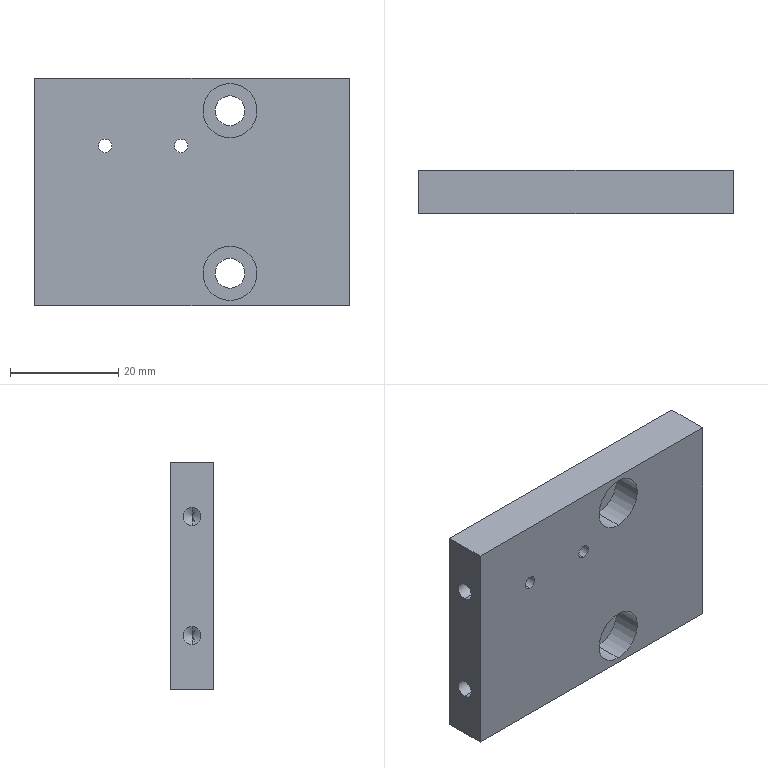Part | SolidWorks | features HoleWzd 3, Extrusion 1 | 1 solid | 28 faces | box 58 x 8 x 42 mm | volume 18259 mm3 | cylinder 16 | plane 8 | cone 4 | commonest cylinder face diameters 2.5 x4 3.3 x4 5.5 x4 10 x4
STEP:
#1=CARTESIAN_POINT('',(-16.,4.,9.75));
#2=VERTEX_POINT('',#1);
#3=CARTESIAN_POINT('',(-16.,4.,7.25));
#4=VERTEX_POINT('',#3);
#5=CARTESIAN_POINT('',(-16.,4.,8.5));
#6=DIRECTION('',(0.,-1.,0.));
#7=DIRECTION('',(0.,0.,-1.));
#8=AXIS2_PLACEMENT_3D('',#5,#6,#7);
#9=CIRCLE('',#8,1.25);
#10=EDGE_CURVE('',#2,#4,#9,.T.);
#11=ORIENTED_EDGE('',*,*,#10,.F.);
#12=CARTESIAN_POINT('',(-16.,-4.,9.75));
#13=VERTEX_POINT('',#12);
#14=CARTESIAN_POINT('',(-16.,-4.,9.75));
#15=DIRECTION('',(0.,-1.,0.));
#16=VECTOR('',#15,1000.);
#17=LINE('',#14,#16);
#18=EDGE_CURVE('',#2,#13,#17,.T.);
#19=ORIENTED_EDGE('',*,*,#18,.T.);
#20=CARTESIAN_POINT('',(-16.,-4.,7.25));
#21=VERTEX_POINT('',#20);
#22=CARTESIAN_POINT('',(-16.,-4.,8.5));
#23=DIRECTION('',(0.,-1.,0.));
#24=DIRECTION('',(0.,0.,-1.));
#25=AXIS2_PLACEMENT_3D('',#22,#23,#24);
#26=CIRCLE('',#25,1.25);
#27=EDGE_CURVE('',#13,#21,#26,.T.);
#28=ORIENTED_EDGE('',*,*,#27,.T.);
#29=CARTESIAN_POINT('',(-16.,-4.,7.25));
#30=DIRECTION('',(0.,-1.,0.));
#31=VECTOR('',#30,1000.);
#32=LINE('',#29,#31);
#33=EDGE_CURVE('',#4,#21,#32,.T.);
#34=ORIENTED_EDGE('',*,*,#33,.F.);
#35=EDGE_LOOP('',(#11,#19,#28,#34));
#36=FACE_OUTER_BOUND('',#35,.T.);
#37=CARTESIAN_POINT('',(-16.,-4.,8.5));
#38=DIRECTION('',(0.,-1.,0.));
#39=DIRECTION('',(0.,0.,-1.));
#40=AXIS2_PLACEMENT_3D('',#37,#38,#39);
#41=CYLINDRICAL_SURFACE('',#40,1.25);
#42=ADVANCED_FACE('',(#36),#41,.F.);
#43=CARTESIAN_POINT('',(-2.,4.,9.75));
#44=VERTEX_POINT('',#43);
#45=CARTESIAN_POINT('',(-2.,4.,7.25));
#46=VERTEX_POINT('',#45);
#47=CARTESIAN_POINT('',(-2.,4.,8.5));
#48=DIRECTION('',(0.,-1.,0.));
#49=DIRECTION('',(0.,0.,-1.));
#50=AXIS2_PLACEMENT_3D('',#47,#48,#49);
#51=CIRCLE('',#50,1.25);
#52=EDGE_CURVE('',#44,#46,#51,.T.);
#53=ORIENTED_EDGE('',*,*,#52,.F.);
#54=CARTESIAN_POINT('',(-2.,-4.,9.75));
#55=VERTEX_POINT('',#54);
#56=CARTESIAN_POINT('',(-2.,-4.,9.75));
#57=DIRECTION('',(0.,-1.,0.));
#58=VECTOR('',#57,1000.);
#59=LINE('',#56,#58);
#60=EDGE_CURVE('',#44,#55,#59,.T.);
#61=ORIENTED_EDGE('',*,*,#60,.T.);
#62=CARTESIAN_POINT('',(-2.,-4.,7.25));
#63=VERTEX_POINT('',#62);
#64=CARTESIAN_POINT('',(-2.,-4.,8.5));
#65=DIRECTION('',(0.,-1.,0.));
#66=DIRECTION('',(0.,0.,-1.));
#67=AXIS2_PLACEMENT_3D('',#64,#65,#66);
#68=CIRCLE('',#67,1.25);
#69=EDGE_CURVE('',#55,#63,#68,.T.);
#70=ORIENTED_EDGE('',*,*,#69,.T.);
#71=CARTESIAN_POINT('',(-2.,-4.,7.25));
#72=DIRECTION('',(0.,-1.,0.));
#73=VECTOR('',#72,1000.);
#74=LINE('',#71,#73);
#75=EDGE_CURVE('',#46,#63,#74,.T.);
#76=ORIENTED_EDGE('',*,*,#75,.F.);
#77=EDGE_LOOP('',(#53,#61,#70,#76));
#78=FACE_OUTER_BOUND('',#77,.T.);
#79=CARTESIAN_POINT('',(-2.,-4.,8.5));
#80=DIRECTION('',(0.,-1.,0.));
#81=DIRECTION('',(0.,0.,-1.));
#82=AXIS2_PLACEMENT_3D('',#79,#80,#81);
#83=CYLINDRICAL_SURFACE('',#82,1.25);
#84=ADVANCED_FACE('',(#78),#83,.F.);
#85=CARTESIAN_POINT('',(-18.9,0.,-12.65));
#86=VERTEX_POINT('',#85);
#87=CARTESIAN_POINT('',(-18.9,0.,-9.35));
#88=VERTEX_POINT('',#87);
#89=CARTESIAN_POINT('',(-18.9,0.,-11.));
#90=DIRECTION('',(-1.,0.,0.));
#91=DIRECTION('',(0.,0.,1.));
#92=AXIS2_PLACEMENT_3D('',#89,#90,#91);
#93=CIRCLE('',#92,1.65);
#94=EDGE_CURVE('',#86,#88,#93,.T.);
#95=ORIENTED_EDGE('',*,*,#94,.F.);
#96=CARTESIAN_POINT('',(-29.,0.,-12.65));
#97=VERTEX_POINT('',#96);
#98=CARTESIAN_POINT('',(-29.,0.,-12.65));
#99=DIRECTION('',(-1.,0.,0.));
#100=VECTOR('',#99,1000.);
#101=LINE('',#98,#100);
#102=EDGE_CURVE('',#86,#97,#101,.T.);
#103=ORIENTED_EDGE('',*,*,#102,.T.);
#104=CARTESIAN_POINT('',(-29.,0.,-9.35));
#105=VERTEX_POINT('',#104);
#106=CARTESIAN_POINT('',(-29.,0.,-11.));
#107=DIRECTION('',(-1.,0.,0.));
#108=DIRECTION('',(0.,0.,1.));
#109=AXIS2_PLACEMENT_3D('',#106,#107,#108);
#110=CIRCLE('',#109,1.65);
#111=EDGE_CURVE('',#97,#105,#110,.T.);
#112=ORIENTED_EDGE('',*,*,#111,.T.);
#113=CARTESIAN_POINT('',(-29.,0.,-9.35));
#114=DIRECTION('',(-1.,0.,0.));
#115=VECTOR('',#114,1000.);
#116=LINE('',#113,#115);
#117=EDGE_CURVE('',#88,#105,#116,.T.);
#118=ORIENTED_EDGE('',*,*,#117,.F.);
#119=EDGE_LOOP('',(#95,#103,#112,#118));
#120=FACE_OUTER_BOUND('',#119,.T.);
#121=CARTESIAN_POINT('',(-29.,0.,-11.));
#122=DIRECTION('',(-1.,0.,0.));
#123=DIRECTION('',(0.,0.,1.));
#124=AXIS2_PLACEMENT_3D('',#121,#122,#123);
#125=CYLINDRICAL_SURFACE('',#124,1.65);
#126=ADVANCED_FACE('',(#120),#125,.F.);
#127=CARTESIAN_POINT('',(-17.909,0.,-11.));
#128=VERTEX_POINT('',#127);
#129=CARTESIAN_POINT('',(-18.9,0.,-9.35));
#130=DIRECTION('',(-0.515,0.,0.8572));
#131=VECTOR('',#130,1000.);
#132=LINE('',#129,#131);
#133=EDGE_CURVE('',#128,#88,#132,.T.);
#134=ORIENTED_EDGE('',*,*,#133,.F.);
#135=CARTESIAN_POINT('',(-18.9,0.,-12.65));
#136=DIRECTION('',(-0.515,0.,-0.8572));
#137=VECTOR('',#136,1000.);
#138=LINE('',#135,#137);
#139=EDGE_CURVE('',#128,#86,#138,.T.);
#140=ORIENTED_EDGE('',*,*,#139,.T.);
#141=ORIENTED_EDGE('',*,*,#94,.T.);
#142=EDGE_LOOP('',(#134,#140,#141));
#143=FACE_OUTER_BOUND('',#142,.T.);
#144=CARTESIAN_POINT('',(-18.9,0.,-11.));
#145=DIRECTION('',(-1.,0.,0.));
#146=DIRECTION('',(0.,0.,1.));
#147=AXIS2_PLACEMENT_3D('',#144,#145,#146);
#148=CONICAL_SURFACE('',#147,1.65,1.03);
#149=ADVANCED_FACE('',(#143),#148,.F.);
#150=CARTESIAN_POINT('',(-18.9,0.,9.35));
#151=VERTEX_POINT('',#150);
#152=CARTESIAN_POINT('',(-18.9,0.,12.65));
#153=VERTEX_POINT('',#152);
#154=CARTESIAN_POINT('',(-18.9,0.,11.));
#155=DIRECTION('',(-1.,0.,0.));
#156=DIRECTION('',(0.,0.,1.));
#157=AXIS2_PLACEMENT_3D('',#154,#155,#156);
#158=CIRCLE('',#157,1.65);
#159=EDGE_CURVE('',#151,#153,#158,.T.);
#160=ORIENTED_EDGE('',*,*,#159,.F.);
#161=CARTESIAN_POINT('',(-29.,0.,9.35));
#162=VERTEX_POINT('',#161);
#163=CARTESIAN_POINT('',(-29.,0.,9.35));
#164=DIRECTION('',(-1.,0.,0.));
#165=VECTOR('',#164,1000.);
#166=LINE('',#163,#165);
#167=EDGE_CURVE('',#151,#162,#166,.T.);
#168=ORIENTED_EDGE('',*,*,#167,.T.);
#169=CARTESIAN_POINT('',(-29.,0.,12.65));
#170=VERTEX_POINT('',#169);
#171=CARTESIAN_POINT('',(-29.,0.,11.));
#172=DIRECTION('',(-1.,0.,0.));
#173=DIRECTION('',(0.,0.,1.));
#174=AXIS2_PLACEMENT_3D('',#171,#172,#173);
#175=CIRCLE('',#174,1.65);
#176=EDGE_CURVE('',#162,#170,#175,.T.);
#177=ORIENTED_EDGE('',*,*,#176,.T.);
#178=CARTESIAN_POINT('',(-29.,0.,12.65));
#179=DIRECTION('',(-1.,0.,0.));
#180=VECTOR('',#179,1000.);
#181=LINE('',#178,#180);
#182=EDGE_CURVE('',#153,#170,#181,.T.);
#183=ORIENTED_EDGE('',*,*,#182,.F.);
#184=EDGE_LOOP('',(#160,#168,#177,#183));
#185=FACE_OUTER_BOUND('',#184,.T.);
#186=CARTESIAN_POINT('',(-29.,0.,11.));
#187=DIRECTION('',(-1.,0.,0.));
#188=DIRECTION('',(0.,0.,1.));
#189=AXIS2_PLACEMENT_3D('',#186,#187,#188);
#190=CYLINDRICAL_SURFACE('',#189,1.65);
#191=ADVANCED_FACE('',(#185),#190,.F.);
#192=CARTESIAN_POINT('',(-17.909,0.,11.));
#193=VERTEX_POINT('',#192);
#194=CARTESIAN_POINT('',(-18.9,0.,12.65));
#195=DIRECTION('',(-0.515,0.,0.8572));
#196=VECTOR('',#195,1000.);
#197=LINE('',#194,#196);
#198=EDGE_CURVE('',#193,#153,#197,.T.);
#199=ORIENTED_EDGE('',*,*,#198,.F.);
#200=CARTESIAN_POINT('',(-18.9,0.,9.35));
#201=DIRECTION('',(-0.515,0.,-0.8572));
#202=VECTOR('',#201,1000.);
#203=LINE('',#200,#202);
#204=EDGE_CURVE('',#193,#151,#203,.T.);
#205=ORIENTED_EDGE('',*,*,#204,.T.);
#206=ORIENTED_EDGE('',*,*,#159,.T.);
#207=EDGE_LOOP('',(#199,#205,#206));
#208=FACE_OUTER_BOUND('',#207,.T.);
#209=CARTESIAN_POINT('',(-18.9,0.,11.));
#210=DIRECTION('',(-1.,0.,0.));
#211=DIRECTION('',(0.,0.,1.));
#212=AXIS2_PLACEMENT_3D('',#209,#210,#211);
#213=CONICAL_SURFACE('',#212,1.65,1.03);
#214=ADVANCED_FACE('',(#208),#213,.F.);
#215=CARTESIAN_POINT('',(7.,1.4,-10.));
#216=VERTEX_POINT('',#215);
#217=CARTESIAN_POINT('',(7.,1.4,-20.));
#218=VERTEX_POINT('',#217);
#219=CARTESIAN_POINT('',(7.,1.4,-15.));
#220=DIRECTION('',(0.,-1.,0.));
#221=DIRECTION('',(0.,0.,-1.));
#222=AXIS2_PLACEMENT_3D('',#219,#220,#221);
#223=CIRCLE('',#222,5.);
#224=EDGE_CURVE('',#216,#218,#223,.T.);
#225=ORIENTED_EDGE('',*,*,#224,.F.);
#226=CARTESIAN_POINT('',(7.,-4.,-10.));
#227=VERTEX_POINT('',#226);
#228=CARTESIAN_POINT('',(7.,-4.,-10.));
#229=DIRECTION('',(0.,-1.,0.));
#230=VECTOR('',#229,1000.);
#231=LINE('',#228,#230);
#232=EDGE_CURVE('',#216,#227,#231,.T.);
#233=ORIENTED_EDGE('',*,*,#232,.T.);
#234=CARTESIAN_POINT('',(7.,-4.,-20.));
#235=VERTEX_POINT('',#234);
#236=CARTESIAN_POINT('',(7.,-4.,-15.));
#237=DIRECTION('',(0.,-1.,0.));
#238=DIRECTION('',(0.,0.,-1.));
#239=AXIS2_PLACEMENT_3D('',#236,#237,#238);
#240=CIRCLE('',#239,5.);
#241=EDGE_CURVE('',#227,#235,#240,.T.);
#242=ORIENTED_EDGE('',*,*,#241,.T.);
#243=CARTESIAN_POINT('',(7.,-4.,-20.));
#244=DIRECTION('',(0.,-1.,0.));
#245=VECTOR('',#244,1000.);
#246=LINE('',#243,#245);
#247=EDGE_CURVE('',#218,#235,#246,.T.);
#248=ORIENTED_EDGE('',*,*,#247,.F.);
#249=EDGE_LOOP('',(#225,#233,#242,#248));
#250=FACE_OUTER_BOUND('',#249,.T.);
#251=CARTESIAN_POINT('',(7.,-4.,-15.));
#252=DIRECTION('',(0.,-1.,0.));
#253=DIRECTION('',(0.,0.,-1.));
#254=AXIS2_PLACEMENT_3D('',#251,#252,#253);
#255=CYLINDRICAL_SURFACE('',#254,5.);
#256=ADVANCED_FACE('',(#250),#255,.F.);
#257=CARTESIAN_POINT('',(7.,4.,-12.25));
#258=VERTEX_POINT('',#257);
#259=CARTESIAN_POINT('',(7.,4.,-17.75));
#260=VERTEX_POINT('',#259);
#261=CARTESIAN_POINT('',(7.,4.,-15.));
#262=DIRECTION('',(0.,-1.,0.));
#263=DIRECTION('',(0.,0.,-1.));
#264=AXIS2_PLACEMENT_3D('',#261,#262,#263);
#265=CIRCLE('',#264,2.75);
#266=EDGE_CURVE('',#258,#260,#265,.T.);
#267=ORIENTED_EDGE('',*,*,#266,.F.);
#268=CARTESIAN_POINT('',(7.,1.4,-12.25));
#269=VERTEX_POINT('',#268);
#270=CARTESIAN_POINT('',(7.,-4.,-12.25));
#271=DIRECTION('',(0.,-1.,0.));
#272=VECTOR('',#271,1000.);
#273=LINE('',#270,#272);
#274=EDGE_CURVE('',#258,#269,#273,.T.);
#275=ORIENTED_EDGE('',*,*,#274,.T.);
#276=CARTESIAN_POINT('',(7.,1.4,-17.75));
#277=VERTEX_POINT('',#276);
#278=CARTESIAN_POINT('',(7.,1.4,-15.));
#279=DIRECTION('',(0.,-1.,0.));
#280=DIRECTION('',(0.,0.,-1.));
#281=AXIS2_PLACEMENT_3D('',#278,#279,#280);
#282=CIRCLE('',#281,2.75);
#283=EDGE_CURVE('',#269,#277,#282,.T.);
#284=ORIENTED_EDGE('',*,*,#283,.T.);
#285=CARTESIAN_POINT('',(7.,-4.,-17.75));
#286=DIRECTION('',(0.,-1.,0.));
#287=VECTOR('',#286,1000.);
#288=LINE('',#285,#287);
#289=EDGE_CURVE('',#260,#277,#288,.T.);
#290=ORIENTED_EDGE('',*,*,#289,.F.);
#291=EDGE_LOOP('',(#267,#275,#284,#290));
#292=FACE_OUTER_BOUND('',#291,.T.);
#293=CARTESIAN_POINT('',(7.,-4.,-15.));
#294=DIRECTION('',(0.,-1.,0.));
#295=DIRECTION('',(0.,0.,-1.));
#296=AXIS2_PLACEMENT_3D('',#293,#294,#295);
#297=CYLINDRICAL_SURFACE('',#296,2.75);
#298=ADVANCED_FACE('',(#292),#297,.F.);
#299=CARTESIAN_POINT('',(7.,1.4,20.));
#300=VERTEX_POINT('',#299);
#301=CARTESIAN_POINT('',(7.,1.4,10.));
#302=VERTEX_POINT('',#301);
#303=CARTESIAN_POINT('',(7.,1.4,15.));
#304=DIRECTION('',(0.,-1.,0.));
#305=DIRECTION('',(0.,0.,-1.));
#306=AXIS2_PLACEMENT_3D('',#303,#304,#305);
#307=CIRCLE('',#306,5.);
#308=EDGE_CURVE('',#300,#302,#307,.T.);
#309=ORIENTED_EDGE('',*,*,#308,.F.);
#310=CARTESIAN_POINT('',(7.,-4.,20.));
#311=VERTEX_POINT('',#310);
#312=CARTESIAN_POINT('',(7.,-4.,20.));
#313=DIRECTION('',(0.,-1.,0.));
#314=VECTOR('',#313,1000.);
#315=LINE('',#312,#314);
#316=EDGE_CURVE('',#300,#311,#315,.T.);
#317=ORIENTED_EDGE('',*,*,#316,.T.);
#318=CARTESIAN_POINT('',(7.,-4.,10.));
#319=VERTEX_POINT('',#318);
#320=CARTESIAN_POINT('',(7.,-4.,15.));
#321=DIRECTION('',(0.,-1.,0.));
#322=DIRECTION('',(0.,0.,-1.));
#323=AXIS2_PLACEMENT_3D('',#320,#321,#322);
#324=CIRCLE('',#323,5.);
#325=EDGE_CURVE('',#311,#319,#324,.T.);
#326=ORIENTED_EDGE('',*,*,#325,.T.);
#327=CARTESIAN_POINT('',(7.,-4.,10.));
#328=DIRECTION('',(0.,-1.,0.));
#329=VECTOR('',#328,1000.);
#330=LINE('',#327,#329);
#331=EDGE_CURVE('',#302,#319,#330,.T.);
#332=ORIENTED_EDGE('',*,*,#331,.F.);
#333=EDGE_LOOP('',(#309,#317,#326,#332));
#334=FACE_OUTER_BOUND('',#333,.T.);
#335=CARTESIAN_POINT('',(7.,-4.,15.));
#336=DIRECTION('',(0.,-1.,0.));
#337=DIRECTION('',(0.,0.,-1.));
#338=AXIS2_PLACEMENT_3D('',#335,#336,#337);
#339=CYLINDRICAL_SURFACE('',#338,5.);
#340=ADVANCED_FACE('',(#334),#339,.F.);
#341=CARTESIAN_POINT('',(7.,4.,17.75));
#342=VERTEX_POINT('',#341);
#343=CARTESIAN_POINT('',(7.,4.,12.25));
#344=VERTEX_POINT('',#343);
#345=CARTESIAN_POINT('',(7.,4.,15.));
#346=DIRECTION('',(0.,-1.,0.));
#347=DIRECTION('',(0.,0.,-1.));
#348=AXIS2_PLACEMENT_3D('',#345,#346,#347);
#349=CIRCLE('',#348,2.75);
#350=EDGE_CURVE('',#342,#344,#349,.T.);
#351=ORIENTED_EDGE('',*,*,#350,.F.);
#352=CARTESIAN_POINT('',(7.,1.4,17.75));
#353=VERTEX_POINT('',#352);
#354=CARTESIAN_POINT('',(7.,-4.,17.75));
#355=DIRECTION('',(0.,-1.,0.));
#356=VECTOR('',#355,1000.);
#357=LINE('',#354,#356);
#358=EDGE_CURVE('',#342,#353,#357,.T.);
#359=ORIENTED_EDGE('',*,*,#358,.T.);
#360=CARTESIAN_POINT('',(7.,1.4,12.25));
#361=VERTEX_POINT('',#360);
#362=CARTESIAN_POINT('',(7.,1.4,15.));
#363=DIRECTION('',(0.,-1.,0.));
#364=DIRECTION('',(0.,0.,-1.));
#365=AXIS2_PLACEMENT_3D('',#362,#363,#364);
#366=CIRCLE('',#365,2.75);
#367=EDGE_CURVE('',#353,#361,#366,.T.);
#368=ORIENTED_EDGE('',*,*,#367,.T.);
#369=CARTESIAN_POINT('',(7.,-4.,12.25));
#370=DIRECTION('',(0.,-1.,0.));
#371=VECTOR('',#370,1000.);
#372=LINE('',#369,#371);
#373=EDGE_CURVE('',#344,#361,#372,.T.);
#374=ORIENTED_EDGE('',*,*,#373,.F.);
#375=EDGE_LOOP('',(#351,#359,#368,#374));
#376=FACE_OUTER_BOUND('',#375,.T.);
#377=CARTESIAN_POINT('',(7.,-4.,15.));
#378=DIRECTION('',(0.,-1.,0.));
#379=DIRECTION('',(0.,0.,-1.));
#380=AXIS2_PLACEMENT_3D('',#377,#378,#379);
#381=CYLINDRICAL_SURFACE('',#380,2.75);
#382=ADVANCED_FACE('',(#376),#381,.F.);
#383=CARTESIAN_POINT('',(29.,-4.,21.));
#384=VERTEX_POINT('',#383);
#385=CARTESIAN_POINT('',(29.,-4.,-21.));
#386=VERTEX_POINT('',#385);
#387=CARTESIAN_POINT('',(29.,-4.,-21.));
#388=DIRECTION('',(0.,0.,-1.));
#389=VECTOR('',#388,1000.);
#390=LINE('',#387,#389);
#391=EDGE_CURVE('',#384,#386,#390,.T.);
#392=ORIENTED_EDGE('',*,*,#391,.T.);
#393=CARTESIAN_POINT('',(29.,4.,-21.));
#394=VERTEX_POINT('',#393);
#395=CARTESIAN_POINT('',(29.,4.,-21.));
#396=DIRECTION('',(0.,-1.,0.));
#397=VECTOR('',#396,1000.);
#398=LINE('',#395,#397);
#399=EDGE_CURVE('',#394,#386,#398,.T.);
#400=ORIENTED_EDGE('',*,*,#399,.F.);
#401=CARTESIAN_POINT('',(29.,4.,21.));
#402=VERTEX_POINT('',#401);
#403=CARTESIAN_POINT('',(29.,4.,-21.));
#404=DIRECTION('',(0.,0.,-1.));
#405=VECTOR('',#404,1000.);
#406=LINE('',#403,#405);
#407=EDGE_CURVE('',#402,#394,#406,.T.);
#408=ORIENTED_EDGE('',*,*,#407,.F.);
#409=CARTESIAN_POINT('',(29.,4.,21.));
#410=DIRECTION('',(0.,-1.,0.));
#411=VECTOR('',#410,1000.);
#412=LINE('',#409,#411);
#413=EDGE_CURVE('',#402,#384,#412,.T.);
#414=ORIENTED_EDGE('',*,*,#413,.T.);
#415=EDGE_LOOP('',(#392,#400,#408,#414));
#416=FACE_OUTER_BOUND('',#415,.T.);
#417=CARTESIAN_POINT('',(29.,4.,-21.));
#418=DIRECTION('',(-1.,0.,0.));
#419=DIRECTION('',(0.,0.,1.));
#420=AXIS2_PLACEMENT_3D('',#417,#418,#419);
#421=PLANE('',#420);
#422=ADVANCED_FACE('',(#416),#421,.F.);
#423=CARTESIAN_POINT('',(-29.,-4.,-21.));
#424=VERTEX_POINT('',#423);
#425=CARTESIAN_POINT('',(-29.,-4.,-21.));
#426=DIRECTION('',(-1.,0.,0.));
#427=VECTOR('',#426,1000.);
#428=LINE('',#425,#427);
#429=EDGE_CURVE('',#386,#424,#428,.T.);
#430=ORIENTED_EDGE('',*,*,#429,.T.);
#431=CARTESIAN_POINT('',(-29.,4.,-21.));
#432=VERTEX_POINT('',#431);
#433=CARTESIAN_POINT('',(-29.,4.,-21.));
#434=DIRECTION('',(0.,-1.,0.));
#435=VECTOR('',#434,1000.);
#436=LINE('',#433,#435);
#437=EDGE_CURVE('',#432,#424,#436,.T.);
#438=ORIENTED_EDGE('',*,*,#437,.F.);
#439=CARTESIAN_POINT('',(-29.,4.,-21.));
#440=DIRECTION('',(-1.,0.,0.));
#441=VECTOR('',#440,1000.);
#442=LINE('',#439,#441);
#443=EDGE_CURVE('',#394,#432,#442,.T.);
#444=ORIENTED_EDGE('',*,*,#443,.F.);
#445=ORIENTED_EDGE('',*,*,#399,.T.);
#446=EDGE_LOOP('',(#430,#438,#444,#445));
#447=FACE_OUTER_BOUND('',#446,.T.);
#448=CARTESIAN_POINT('',(-29.,4.,-21.));
#449=DIRECTION('',(0.,0.,1.));
#450=DIRECTION('',(1.,0.,0.));
#451=AXIS2_PLACEMENT_3D('',#448,#449,#450);
#452=PLANE('',#451);
#453=ADVANCED_FACE('',(#447),#452,.F.);
#454=CARTESIAN_POINT('',(-29.,0.,-11.));
#455=DIRECTION('',(-1.,0.,0.));
#456=DIRECTION('',(0.,0.,1.));
#457=AXIS2_PLACEMENT_3D('',#454,#455,#456);
#458=CIRCLE('',#457,1.65);
#459=EDGE_CURVE('',#105,#97,#458,.T.);
#460=ORIENTED_EDGE('',*,*,#459,.F.);
#461=ORIENTED_EDGE('',*,*,#111,.F.);
#462=EDGE_LOOP('',(#460,#461));
#463=FACE_BOUND('',#462,.T.);
#464=CARTESIAN_POINT('',(-29.,0.,11.));
#465=DIRECTION('',(-1.,0.,0.));
#466=DIRECTION('',(0.,0.,1.));
#467=AXIS2_PLACEMENT_3D('',#464,#465,#466);
#468=CIRCLE('',#467,1.65);
#469=EDGE_CURVE('',#170,#162,#468,.T.);
#470=ORIENTED_EDGE('',*,*,#469,.F.);
#471=ORIENTED_EDGE('',*,*,#176,.F.);
#472=EDGE_LOOP('',(#470,#471));
#473=FACE_BOUND('',#472,.T.);
#474=CARTESIAN_POINT('',(-29.,-4.,21.));
#475=VERTEX_POINT('',#474);
#476=CARTESIAN_POINT('',(-29.,-4.,-21.));
#477=DIRECTION('',(0.,0.,1.));
#478=VECTOR('',#477,1000.);
#479=LINE('',#476,#478);
#480=EDGE_CURVE('',#424,#475,#479,.T.);
#481=ORIENTED_EDGE('',*,*,#480,.T.);
#482=CARTESIAN_POINT('',(-29.,4.,21.));
#483=VERTEX_POINT('',#482);
#484=CARTESIAN_POINT('',(-29.,4.,21.));
#485=DIRECTION('',(0.,-1.,0.));
#486=VECTOR('',#485,1000.);
#487=LINE('',#484,#486);
#488=EDGE_CURVE('',#483,#475,#487,.T.);
#489=ORIENTED_EDGE('',*,*,#488,.F.);
#490=CARTESIAN_POINT('',(-29.,4.,-21.));
#491=DIRECTION('',(0.,0.,1.));
#492=VECTOR('',#491,1000.);
#493=LINE('',#490,#492);
#494=EDGE_CURVE('',#432,#483,#493,.T.);
#495=ORIENTED_EDGE('',*,*,#494,.F.);
#496=ORIENTED_EDGE('',*,*,#437,.T.);
#497=EDGE_LOOP('',(#481,#489,#495,#496));
#498=FACE_OUTER_BOUND('',#497,.T.);
#499=CARTESIAN_POINT('',(-29.,4.,-21.));
#500=DIRECTION('',(1.,0.,0.));
#501=DIRECTION('',(0.,0.,-1.));
#502=AXIS2_PLACEMENT_3D('',#499,#500,#501);
#503=PLANE('',#502);
#504=ADVANCED_FACE('',(#463,#473,#498),#503,.F.);
#505=CARTESIAN_POINT('',(-29.,-4.,21.));
#506=DIRECTION('',(1.,0.,0.));
#507=VECTOR('',#506,1000.);
#508=LINE('',#505,#507);
#509=EDGE_CURVE('',#475,#384,#508,.T.);
#510=ORIENTED_EDGE('',*,*,#509,.T.);
#511=ORIENTED_EDGE('',*,*,#413,.F.);
#512=CARTESIAN_POINT('',(-29.,4.,21.));
#513=DIRECTION('',(1.,0.,0.));
#514=VECTOR('',#513,1000.);
#515=LINE('',#512,#514);
#516=EDGE_CURVE('',#483,#402,#515,.T.);
#517=ORIENTED_EDGE('',*,*,#516,.F.);
#518=ORIENTED_EDGE('',*,*,#488,.T.);
#519=EDGE_LOOP('',(#510,#511,#517,#518));
#520=FACE_OUTER_BOUND('',#519,.T.);
#521=CARTESIAN_POINT('',(-29.,4.,21.));
#522=DIRECTION('',(0.,0.,-1.));
#523=DIRECTION('',(-1.,0.,0.));
#524=AXIS2_PLACEMENT_3D('',#521,#522,#523);
#525=PLANE('',#524);
#526=ADVANCED_FACE('',(#520),#525,.F.);
#527=CARTESIAN_POINT('',(-16.,4.,8.5));
#528=DIRECTION('',(0.,-1.,0.));
#529=DIRECTION('',(0.,0.,-1.));
#530=AXIS2_PLACEMENT_3D('',#527,#528,#529);
#531=CIRCLE('',#530,1.25);
#532=EDGE_CURVE('',#4,#2,#531,.T.);
#533=ORIENTED_EDGE('',*,*,#532,.T.);
#534=ORIENTED_EDGE('',*,*,#10,.T.);
#535=EDGE_LOOP('',(#533,#534));
#536=FACE_BOUND('',#535,.T.);
#537=CARTESIAN_POINT('',(-2.,4.,8.5));
#538=DIRECTION('',(0.,-1.,0.));
#539=DIRECTION('',(0.,0.,-1.));
#540=AXIS2_PLACEMENT_3D('',#537,#538,#539);
#541=CIRCLE('',#540,1.25);
#542=EDGE_CURVE('',#46,#44,#541,.T.);
#543=ORIENTED_EDGE('',*,*,#542,.T.);
#544=ORIENTED_EDGE('',*,*,#52,.T.);
#545=EDGE_LOOP('',(#543,#544));
#546=FACE_BOUND('',#545,.T.);
#547=CARTESIAN_POINT('',(7.,4.,-15.));
#548=DIRECTION('',(0.,-1.,0.));
#549=DIRECTION('',(0.,0.,-1.));
#550=AXIS2_PLACEMENT_3D('',#547,#548,#549);
#551=CIRCLE('',#550,2.75);
#552=EDGE_CURVE('',#260,#258,#551,.T.);
#553=ORIENTED_EDGE('',*,*,#552,.T.);
#554=ORIENTED_EDGE('',*,*,#266,.T.);
#555=EDGE_LOOP('',(#553,#554));
#556=FACE_BOUND('',#555,.T.);
#557=CARTESIAN_POINT('',(7.,4.,15.));
#558=DIRECTION('',(0.,-1.,0.));
#559=DIRECTION('',(0.,0.,-1.));
#560=AXIS2_PLACEMENT_3D('',#557,#558,#559);
#561=CIRCLE('',#560,2.75);
#562=EDGE_CURVE('',#344,#342,#561,.T.);
#563=ORIENTED_EDGE('',*,*,#562,.T.);
#564=ORIENTED_EDGE('',*,*,#350,.T.);
#565=EDGE_LOOP('',(#563,#564));
#566=FACE_BOUND('',#565,.T.);
#567=ORIENTED_EDGE('',*,*,#407,.T.);
#568=ORIENTED_EDGE('',*,*,#443,.T.);
#569=ORIENTED_EDGE('',*,*,#494,.T.);
#570=ORIENTED_EDGE('',*,*,#516,.T.);
#571=EDGE_LOOP('',(#567,#568,#569,#570));
#572=FACE_OUTER_BOUND('',#571,.T.);
#573=CARTESIAN_POINT('',(0.,4.,0.));
#574=DIRECTION('',(0.,1.,0.));
#575=DIRECTION('',(0.,0.,1.));
#576=AXIS2_PLACEMENT_3D('',#573,#574,#575);
#577=PLANE('',#576);
#578=ADVANCED_FACE('',(#536,#546,#556,#566,#572),#577,.T.);
#579=CARTESIAN_POINT('',(-16.,-4.,8.5));
#580=DIRECTION('',(0.,-1.,0.));
#581=DIRECTION('',(0.,0.,-1.));
#582=AXIS2_PLACEMENT_3D('',#579,#580,#581);
#583=CIRCLE('',#582,1.25);
#584=EDGE_CURVE('',#21,#13,#583,.T.);
#585=ORIENTED_EDGE('',*,*,#584,.F.);
#586=ORIENTED_EDGE('',*,*,#27,.F.);
#587=EDGE_LOOP('',(#585,#586));
#588=FACE_BOUND('',#587,.T.);
#589=CARTESIAN_POINT('',(-2.,-4.,8.5));
#590=DIRECTION('',(0.,-1.,0.));
#591=DIRECTION('',(0.,0.,-1.));
#592=AXIS2_PLACEMENT_3D('',#589,#590,#591);
#593=CIRCLE('',#592,1.25);
#594=EDGE_CURVE('',#63,#55,#593,.T.);
#595=ORIENTED_EDGE('',*,*,#594,.F.);
#596=ORIENTED_EDGE('',*,*,#69,.F.);
#597=EDGE_LOOP('',(#595,#596));
#598=FACE_BOUND('',#597,.T.);
#599=CARTESIAN_POINT('',(7.,-4.,-15.));
#600=DIRECTION('',(0.,-1.,0.));
#601=DIRECTION('',(0.,0.,-1.));
#602=AXIS2_PLACEMENT_3D('',#599,#600,#601);
#603=CIRCLE('',#602,5.);
#604=EDGE_CURVE('',#235,#227,#603,.T.);
#605=ORIENTED_EDGE('',*,*,#604,.F.);
#606=ORIENTED_EDGE('',*,*,#241,.F.);
#607=EDGE_LOOP('',(#605,#606));
#608=FACE_BOUND('',#607,.T.);
#609=CARTESIAN_POINT('',(7.,-4.,15.));
#610=DIRECTION('',(0.,-1.,0.));
#611=DIRECTION('',(0.,0.,-1.));
#612=AXIS2_PLACEMENT_3D('',#609,#610,#611);
#613=CIRCLE('',#612,5.);
#614=EDGE_CURVE('',#319,#311,#613,.T.);
#615=ORIENTED_EDGE('',*,*,#614,.F.);
#616=ORIENTED_EDGE('',*,*,#325,.F.);
#617=EDGE_LOOP('',(#615,#616));
#618=FACE_BOUND('',#617,.T.);
#619=ORIENTED_EDGE('',*,*,#391,.F.);
#620=ORIENTED_EDGE('',*,*,#509,.F.);
#621=ORIENTED_EDGE('',*,*,#480,.F.);
#622=ORIENTED_EDGE('',*,*,#429,.F.);
#623=EDGE_LOOP('',(#619,#620,#621,#622));
#624=FACE_OUTER_BOUND('',#623,.T.);
#625=CARTESIAN_POINT('',(0.,-4.,0.));
#626=DIRECTION('',(0.,1.,0.));
#627=DIRECTION('',(0.,0.,1.));
#628=AXIS2_PLACEMENT_3D('',#625,#626,#627);
#629=PLANE('',#628);
#630=ADVANCED_FACE('',(#588,#598,#608,#618,#624),#629,.F.);
#631=ORIENTED_EDGE('',*,*,#358,.F.);
#632=ORIENTED_EDGE('',*,*,#562,.F.);
#633=ORIENTED_EDGE('',*,*,#373,.T.);
#634=CARTESIAN_POINT('',(7.,1.4,15.));
#635=DIRECTION('',(0.,-1.,0.));
#636=DIRECTION('',(0.,0.,-1.));
#637=AXIS2_PLACEMENT_3D('',#634,#635,#636);
#638=CIRCLE('',#637,2.75);
#639=EDGE_CURVE('',#361,#353,#638,.T.);
#640=ORIENTED_EDGE('',*,*,#639,.T.);
#641=EDGE_LOOP('',(#631,#632,#633,#640));
#642=FACE_OUTER_BOUND('',#641,.T.);
#643=CARTESIAN_POINT('',(7.,-4.,15.));
#644=DIRECTION('',(0.,-1.,0.));
#645=DIRECTION('',(0.,0.,-1.));
#646=AXIS2_PLACEMENT_3D('',#643,#644,#645);
#647=CYLINDRICAL_SURFACE('',#646,2.75);
#648=ADVANCED_FACE('',(#642),#647,.F.);
#649=ORIENTED_EDGE('',*,*,#639,.F.);
#650=ORIENTED_EDGE('',*,*,#367,.F.);
#651=EDGE_LOOP('',(#649,#650));
#652=FACE_BOUND('',#651,.T.);
#653=CARTESIAN_POINT('',(7.,1.4,15.));
#654=DIRECTION('',(0.,-1.,0.));
#655=DIRECTION('',(0.,0.,-1.));
#656=AXIS2_PLACEMENT_3D('',#653,#654,#655);
#657=CIRCLE('',#656,5.);
#658=EDGE_CURVE('',#302,#300,#657,.T.);
#659=ORIENTED_EDGE('',*,*,#658,.T.);
#660=ORIENTED_EDGE('',*,*,#308,.T.);
#661=EDGE_LOOP('',(#659,#660));
#662=FACE_OUTER_BOUND('',#661,.T.);
#663=CARTESIAN_POINT('',(9.75,1.4,15.));
#664=DIRECTION('',(0.,1.,0.));
#665=DIRECTION('',(0.,0.,1.));
#666=AXIS2_PLACEMENT_3D('',#663,#664,#665);
#667=PLANE('',#666);
#668=ADVANCED_FACE('',(#652,#662),#667,.F.);
#669=ORIENTED_EDGE('',*,*,#316,.F.);
#670=ORIENTED_EDGE('',*,*,#658,.F.);
#671=ORIENTED_EDGE('',*,*,#331,.T.);
#672=ORIENTED_EDGE('',*,*,#614,.T.);
#673=EDGE_LOOP('',(#669,#670,#671,#672));
#674=FACE_OUTER_BOUND('',#673,.T.);
#675=CARTESIAN_POINT('',(7.,-4.,15.));
#676=DIRECTION('',(0.,-1.,0.));
#677=DIRECTION('',(0.,0.,-1.));
#678=AXIS2_PLACEMENT_3D('',#675,#676,#677);
#679=CYLINDRICAL_SURFACE('',#678,5.);
#680=ADVANCED_FACE('',(#674),#679,.F.);
#681=ORIENTED_EDGE('',*,*,#274,.F.);
#682=ORIENTED_EDGE('',*,*,#552,.F.);
#683=ORIENTED_EDGE('',*,*,#289,.T.);
#684=CARTESIAN_POINT('',(7.,1.4,-15.));
#685=DIRECTION('',(0.,-1.,0.));
#686=DIRECTION('',(0.,0.,-1.));
#687=AXIS2_PLACEMENT_3D('',#684,#685,#686);
#688=CIRCLE('',#687,2.75);
#689=EDGE_CURVE('',#277,#269,#688,.T.);
#690=ORIENTED_EDGE('',*,*,#689,.T.);
#691=EDGE_LOOP('',(#681,#682,#683,#690));
#692=FACE_OUTER_BOUND('',#691,.T.);
#693=CARTESIAN_POINT('',(7.,-4.,-15.));
#694=DIRECTION('',(0.,-1.,0.));
#695=DIRECTION('',(0.,0.,-1.));
#696=AXIS2_PLACEMENT_3D('',#693,#694,#695);
#697=CYLINDRICAL_SURFACE('',#696,2.75);
#698=ADVANCED_FACE('',(#692),#697,.F.);
#699=ORIENTED_EDGE('',*,*,#689,.F.);
#700=ORIENTED_EDGE('',*,*,#283,.F.);
#701=EDGE_LOOP('',(#699,#700));
#702=FACE_BOUND('',#701,.T.);
#703=CARTESIAN_POINT('',(7.,1.4,-15.));
#704=DIRECTION('',(0.,-1.,0.));
#705=DIRECTION('',(0.,0.,-1.));
#706=AXIS2_PLACEMENT_3D('',#703,#704,#705);
#707=CIRCLE('',#706,5.);
#708=EDGE_CURVE('',#218,#216,#707,.T.);
#709=ORIENTED_EDGE('',*,*,#708,.T.);
#710=ORIENTED_EDGE('',*,*,#224,.T.);
#711=EDGE_LOOP('',(#709,#710));
#712=FACE_OUTER_BOUND('',#711,.T.);
#713=CARTESIAN_POINT('',(9.75,1.4,-15.));
#714=DIRECTION('',(0.,1.,0.));
#715=DIRECTION('',(0.,0.,1.));
#716=AXIS2_PLACEMENT_3D('',#713,#714,#715);
#717=PLANE('',#716);
#718=ADVANCED_FACE('',(#702,#712),#717,.F.);
#719=ORIENTED_EDGE('',*,*,#232,.F.);
#720=ORIENTED_EDGE('',*,*,#708,.F.);
#721=ORIENTED_EDGE('',*,*,#247,.T.);
#722=ORIENTED_EDGE('',*,*,#604,.T.);
#723=EDGE_LOOP('',(#719,#720,#721,#722));
#724=FACE_OUTER_BOUND('',#723,.T.);
#725=CARTESIAN_POINT('',(7.,-4.,-15.));
#726=DIRECTION('',(0.,-1.,0.));
#727=DIRECTION('',(0.,0.,-1.));
#728=AXIS2_PLACEMENT_3D('',#725,#726,#727);
#729=CYLINDRICAL_SURFACE('',#728,5.);
#730=ADVANCED_FACE('',(#724),#729,.F.);
#731=ORIENTED_EDGE('',*,*,#204,.F.);
#732=ORIENTED_EDGE('',*,*,#198,.T.);
#733=CARTESIAN_POINT('',(-18.9,0.,11.));
#734=DIRECTION('',(-1.,0.,0.));
#735=DIRECTION('',(0.,0.,1.));
#736=AXIS2_PLACEMENT_3D('',#733,#734,#735);
#737=CIRCLE('',#736,1.65);
#738=EDGE_CURVE('',#153,#151,#737,.T.);
#739=ORIENTED_EDGE('',*,*,#738,.T.);
#740=EDGE_LOOP('',(#731,#732,#739));
#741=FACE_OUTER_BOUND('',#740,.T.);
#742=CARTESIAN_POINT('',(-18.9,0.,11.));
#743=DIRECTION('',(-1.,0.,0.));
#744=DIRECTION('',(0.,0.,1.));
#745=AXIS2_PLACEMENT_3D('',#742,#743,#744);
#746=CONICAL_SURFACE('',#745,1.65,1.03);
#747=ADVANCED_FACE('',(#741),#746,.F.);
#748=ORIENTED_EDGE('',*,*,#167,.F.);
#749=ORIENTED_EDGE('',*,*,#738,.F.);
#750=ORIENTED_EDGE('',*,*,#182,.T.);
#751=ORIENTED_EDGE('',*,*,#469,.T.);
#752=EDGE_LOOP('',(#748,#749,#750,#751));
#753=FACE_OUTER_BOUND('',#752,.T.);
#754=CARTESIAN_POINT('',(-29.,0.,11.));
#755=DIRECTION('',(-1.,0.,0.));
#756=DIRECTION('',(0.,0.,1.));
#757=AXIS2_PLACEMENT_3D('',#754,#755,#756);
#758=CYLINDRICAL_SURFACE('',#757,1.65);
#759=ADVANCED_FACE('',(#753),#758,.F.);
#760=ORIENTED_EDGE('',*,*,#139,.F.);
#761=ORIENTED_EDGE('',*,*,#133,.T.);
#762=CARTESIAN_POINT('',(-18.9,0.,-11.));
#763=DIRECTION('',(-1.,0.,0.));
#764=DIRECTION('',(0.,0.,1.));
#765=AXIS2_PLACEMENT_3D('',#762,#763,#764);
#766=CIRCLE('',#765,1.65);
#767=EDGE_CURVE('',#88,#86,#766,.T.);
#768=ORIENTED_EDGE('',*,*,#767,.T.);
#769=EDGE_LOOP('',(#760,#761,#768));
#770=FACE_OUTER_BOUND('',#769,.T.);
#771=CARTESIAN_POINT('',(-18.9,0.,-11.));
#772=DIRECTION('',(-1.,0.,0.));
#773=DIRECTION('',(0.,0.,1.));
#774=AXIS2_PLACEMENT_3D('',#771,#772,#773);
#775=CONICAL_SURFACE('',#774,1.65,1.03);
#776=ADVANCED_FACE('',(#770),#775,.F.);
#777=ORIENTED_EDGE('',*,*,#102,.F.);
#778=ORIENTED_EDGE('',*,*,#767,.F.);
#779=ORIENTED_EDGE('',*,*,#117,.T.);
#780=ORIENTED_EDGE('',*,*,#459,.T.);
#781=EDGE_LOOP('',(#777,#778,#779,#780));
#782=FACE_OUTER_BOUND('',#781,.T.);
#783=CARTESIAN_POINT('',(-29.,0.,-11.));
#784=DIRECTION('',(-1.,0.,0.));
#785=DIRECTION('',(0.,0.,1.));
#786=AXIS2_PLACEMENT_3D('',#783,#784,#785);
#787=CYLINDRICAL_SURFACE('',#786,1.65);
#788=ADVANCED_FACE('',(#782),#787,.F.);
#789=ORIENTED_EDGE('',*,*,#60,.F.);
#790=ORIENTED_EDGE('',*,*,#542,.F.);
#791=ORIENTED_EDGE('',*,*,#75,.T.);
#792=ORIENTED_EDGE('',*,*,#594,.T.);
#793=EDGE_LOOP('',(#789,#790,#791,#792));
#794=FACE_OUTER_BOUND('',#793,.T.);
#795=CARTESIAN_POINT('',(-2.,-4.,8.5));
#796=DIRECTION('',(0.,-1.,0.));
#797=DIRECTION('',(0.,0.,-1.));
#798=AXIS2_PLACEMENT_3D('',#795,#796,#797);
#799=CYLINDRICAL_SURFACE('',#798,1.25);
#800=ADVANCED_FACE('',(#794),#799,.F.);
#801=ORIENTED_EDGE('',*,*,#18,.F.);
#802=ORIENTED_EDGE('',*,*,#532,.F.);
#803=ORIENTED_EDGE('',*,*,#33,.T.);
#804=ORIENTED_EDGE('',*,*,#584,.T.);
#805=EDGE_LOOP('',(#801,#802,#803,#804));
#806=FACE_OUTER_BOUND('',#805,.T.);
#807=CARTESIAN_POINT('',(-16.,-4.,8.5));
#808=DIRECTION('',(0.,-1.,0.));
#809=DIRECTION('',(0.,0.,-1.));
#810=AXIS2_PLACEMENT_3D('',#807,#808,#809);
#811=CYLINDRICAL_SURFACE('',#810,1.25);
#812=ADVANCED_FACE('',(#806),#811,.F.);
#813=CLOSED_SHELL('',(#42,#84,#126,#149,#191,#214,#256,#298,#340,#382,#422,#453,#504,#526,#578,#630,#648,#668,#680,#698,#718,#730,#747,#759,#776,#788,#800,#812));
#814=MANIFOLD_SOLID_BREP('',#813);
#815=CARTESIAN_POINT('',(0.,0.,0.));
#816=DIRECTION('',(0.,0.,1.));
#817=DIRECTION('',(1.,0.,0.));
#818=AXIS2_PLACEMENT_3D('',#815,#816,#817);
#819=(LENGTH_UNIT()NAMED_UNIT(*)SI_UNIT(.MILLI.,.METRE.));
#820=UNCERTAINTY_MEASURE_WITH_UNIT(LENGTH_MEASURE(0.00001),#819,'','');
#821=(NAMED_UNIT(*)PLANE_ANGLE_UNIT()SI_UNIT($,.RADIAN.));
#822=(NAMED_UNIT(*)SI_UNIT($,.STERADIAN.)SOLID_ANGLE_UNIT());
#823=(GEOMETRIC_REPRESENTATION_CONTEXT(3)GLOBAL_UNCERTAINTY_ASSIGNED_CONTEXT((#820))GLOBAL_UNIT_ASSIGNED_CONTEXT((#819,#821,#822))REPRESENTATION_CONTEXT('',''));
#824=ADVANCED_BREP_SHAPE_REPRESENTATION('',(#814,#818),#823);